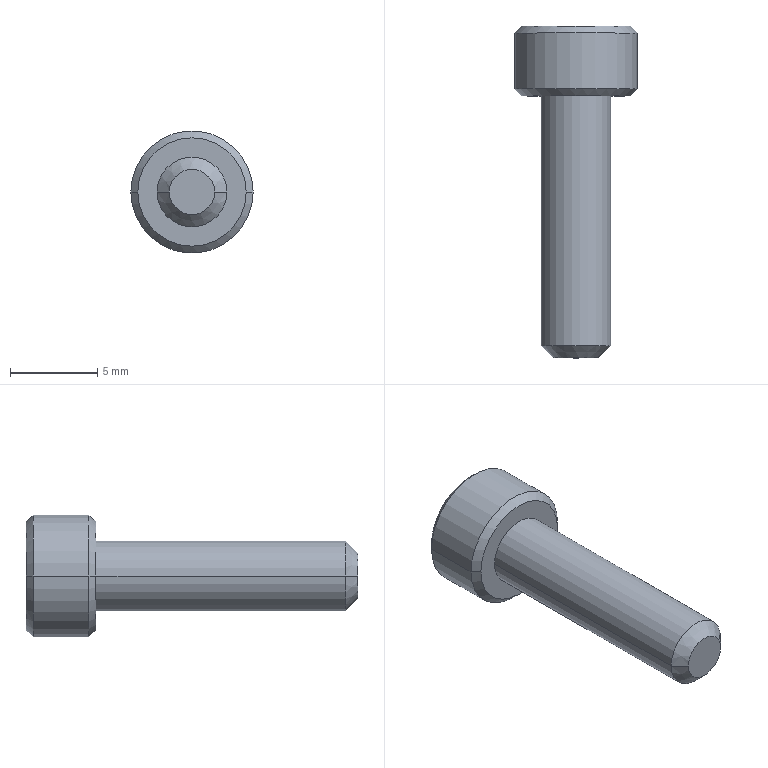Part | STEP file | BB62-M4-15L-12 | 1 solid | 27 faces | box 7 x 19 x 7 mm | volume 317.881 mm3 | plane 15 | cone 8 | cylinder 4 | commonest cylinder face diameters 4 x2 7 x2
STEP:
#1=CARTESIAN_POINT('',(0.,1.007,0.));
#2=VERTEX_POINT('',#1);
#3=CARTESIAN_POINT('',(1.72,2.,0.));
#4=VERTEX_POINT('',#3);
#5=CARTESIAN_POINT('',(0.,1.007,0.));
#6=DIRECTION('',(0.866,0.5,0.));
#7=VECTOR('',#6,1000.);
#8=LINE('',#5,#7);
#9=EDGE_CURVE('',#2,#4,#8,.T.);
#10=ORIENTED_EDGE('',*,*,#9,.F.);
#11=CARTESIAN_POINT('',(-1.72,2.,0.));
#12=VERTEX_POINT('',#11);
#13=CARTESIAN_POINT('',(0.,1.007,0.));
#14=DIRECTION('',(-0.866,0.5,0.));
#15=VECTOR('',#14,1000.);
#16=LINE('',#13,#15);
#17=EDGE_CURVE('',#2,#12,#16,.T.);
#18=ORIENTED_EDGE('',*,*,#17,.T.);
#19=CARTESIAN_POINT('',(-1.49,2.,0.86));
#20=VERTEX_POINT('',#19);
#21=CARTESIAN_POINT('',(0.,2.,0.));
#22=DIRECTION('',(0.,-1.,0.));
#23=DIRECTION('',(-1.,0.,0.));
#24=AXIS2_PLACEMENT_3D('',#21,#22,#23);
#25=CIRCLE('',#24,1.72);
#26=EDGE_CURVE('',#20,#12,#25,.T.);
#27=ORIENTED_EDGE('',*,*,#26,.F.);
#28=CARTESIAN_POINT('',(0.,2.,1.72));
#29=VERTEX_POINT('',#28);
#30=CARTESIAN_POINT('',(0.,2.,0.));
#31=DIRECTION('',(0.,-1.,0.));
#32=DIRECTION('',(-1.,0.,0.));
#33=AXIS2_PLACEMENT_3D('',#30,#31,#32);
#34=CIRCLE('',#33,1.72);
#35=EDGE_CURVE('',#29,#20,#34,.T.);
#36=ORIENTED_EDGE('',*,*,#35,.F.);
#37=CARTESIAN_POINT('',(1.49,2.,0.86));
#38=VERTEX_POINT('',#37);
#39=CARTESIAN_POINT('',(0.,2.,0.));
#40=DIRECTION('',(0.,-1.,0.));
#41=DIRECTION('',(-1.,0.,0.));
#42=AXIS2_PLACEMENT_3D('',#39,#40,#41);
#43=CIRCLE('',#42,1.72);
#44=EDGE_CURVE('',#38,#29,#43,.T.);
#45=ORIENTED_EDGE('',*,*,#44,.F.);
#46=CARTESIAN_POINT('',(0.,2.,0.));
#47=DIRECTION('',(0.,-1.,0.));
#48=DIRECTION('',(-1.,0.,0.));
#49=AXIS2_PLACEMENT_3D('',#46,#47,#48);
#50=CIRCLE('',#49,1.72);
#51=EDGE_CURVE('',#4,#38,#50,.T.);
#52=ORIENTED_EDGE('',*,*,#51,.F.);
#53=EDGE_LOOP('',(#10,#18,#27,#36,#45,#52));
#54=FACE_OUTER_BOUND('',#53,.T.);
#55=CARTESIAN_POINT('',(0.,1001.007,0.));
#56=DIRECTION('',(0.,1.,0.));
#57=DIRECTION('',(1.,0.,0.));
#58=AXIS2_PLACEMENT_3D('',#55,#56,#57);
#59=CONICAL_SURFACE('',#58,1732.051,1.047);
#60=ADVANCED_FACE('',(#54),#59,.F.);
#61=CARTESIAN_POINT('',(1.3,-15.,0.));
#62=VERTEX_POINT('',#61);
#63=CARTESIAN_POINT('',(-1.3,-15.,0.));
#64=VERTEX_POINT('',#63);
#65=CARTESIAN_POINT('',(0.,-15.,0.));
#66=DIRECTION('',(0.,1.,0.));
#67=DIRECTION('',(1.,0.,0.));
#68=AXIS2_PLACEMENT_3D('',#65,#66,#67);
#69=CIRCLE('',#68,1.3);
#70=EDGE_CURVE('',#62,#64,#69,.T.);
#71=ORIENTED_EDGE('',*,*,#70,.T.);
#72=CARTESIAN_POINT('',(-2.,-14.3,0.));
#73=VERTEX_POINT('',#72);
#74=CARTESIAN_POINT('',(-1.3,-15.,0.));
#75=DIRECTION('',(-0.7071,0.7071,0.));
#76=VECTOR('',#75,1000.);
#77=LINE('',#74,#76);
#78=EDGE_CURVE('',#64,#73,#77,.T.);
#79=ORIENTED_EDGE('',*,*,#78,.T.);
#80=CARTESIAN_POINT('',(2.,-14.3,0.));
#81=VERTEX_POINT('',#80);
#82=CARTESIAN_POINT('',(0.,-14.3,0.));
#83=DIRECTION('',(0.,-1.,0.));
#84=DIRECTION('',(-1.,0.,0.));
#85=AXIS2_PLACEMENT_3D('',#82,#83,#84);
#86=CIRCLE('',#85,2.);
#87=EDGE_CURVE('',#73,#81,#86,.T.);
#88=ORIENTED_EDGE('',*,*,#87,.T.);
#89=CARTESIAN_POINT('',(1.3,-15.,0.));
#90=DIRECTION('',(0.7071,0.7071,0.));
#91=VECTOR('',#90,1000.);
#92=LINE('',#89,#91);
#93=EDGE_CURVE('',#62,#81,#92,.T.);
#94=ORIENTED_EDGE('',*,*,#93,.F.);
#95=EDGE_LOOP('',(#71,#79,#88,#94));
#96=FACE_OUTER_BOUND('',#95,.T.);
#97=CARTESIAN_POINT('',(0.,-15.,0.));
#98=DIRECTION('',(0.,1.,0.));
#99=DIRECTION('',(1.,0.,0.));
#100=AXIS2_PLACEMENT_3D('',#97,#98,#99);
#101=CONICAL_SURFACE('',#100,1.3,0.7854);
#102=ADVANCED_FACE('',(#96),#101,.T.);
#103=ORIENTED_EDGE('',*,*,#87,.F.);
#104=CARTESIAN_POINT('',(-2.,0.,0.));
#105=VERTEX_POINT('',#104);
#106=CARTESIAN_POINT('',(-2.,-14.3,0.));
#107=DIRECTION('',(0.,1.,0.));
#108=VECTOR('',#107,1000.);
#109=LINE('',#106,#108);
#110=EDGE_CURVE('',#73,#105,#109,.T.);
#111=ORIENTED_EDGE('',*,*,#110,.T.);
#112=CARTESIAN_POINT('',(2.,0.,0.));
#113=VERTEX_POINT('',#112);
#114=CARTESIAN_POINT('',(0.,0.,0.));
#115=DIRECTION('',(0.,-1.,0.));
#116=DIRECTION('',(-1.,0.,0.));
#117=AXIS2_PLACEMENT_3D('',#114,#115,#116);
#118=CIRCLE('',#117,2.);
#119=EDGE_CURVE('',#105,#113,#118,.T.);
#120=ORIENTED_EDGE('',*,*,#119,.T.);
#121=CARTESIAN_POINT('',(2.,-14.3,0.));
#122=DIRECTION('',(0.,1.,0.));
#123=VECTOR('',#122,1000.);
#124=LINE('',#121,#123);
#125=EDGE_CURVE('',#81,#113,#124,.T.);
#126=ORIENTED_EDGE('',*,*,#125,.F.);
#127=EDGE_LOOP('',(#103,#111,#120,#126));
#128=FACE_OUTER_BOUND('',#127,.T.);
#129=CARTESIAN_POINT('',(0.,-14.3,0.));
#130=DIRECTION('',(0.,1.,0.));
#131=DIRECTION('',(1.,0.,0.));
#132=AXIS2_PLACEMENT_3D('',#129,#130,#131);
#133=CYLINDRICAL_SURFACE('',#132,2.);
#134=ADVANCED_FACE('',(#128),#133,.T.);
#135=CARTESIAN_POINT('',(-3.1,4.,0.));
#136=VERTEX_POINT('',#135);
#137=CARTESIAN_POINT('',(3.1,4.,0.));
#138=VERTEX_POINT('',#137);
#139=CARTESIAN_POINT('',(0.,4.,0.));
#140=DIRECTION('',(0.,-1.,0.));
#141=DIRECTION('',(-1.,0.,0.));
#142=AXIS2_PLACEMENT_3D('',#139,#140,#141);
#143=CIRCLE('',#142,3.1);
#144=EDGE_CURVE('',#136,#138,#143,.T.);
#145=ORIENTED_EDGE('',*,*,#144,.T.);
#146=CARTESIAN_POINT('',(3.5,3.6,0.));
#147=VERTEX_POINT('',#146);
#148=CARTESIAN_POINT('',(3.5,3.6,0.));
#149=DIRECTION('',(0.7071,-0.7071,0.));
#150=VECTOR('',#149,1000.);
#151=LINE('',#148,#150);
#152=EDGE_CURVE('',#138,#147,#151,.T.);
#153=ORIENTED_EDGE('',*,*,#152,.T.);
#154=CARTESIAN_POINT('',(-3.5,3.6,0.));
#155=VERTEX_POINT('',#154);
#156=CARTESIAN_POINT('',(0.,3.6,0.));
#157=DIRECTION('',(0.,-1.,0.));
#158=DIRECTION('',(-1.,0.,0.));
#159=AXIS2_PLACEMENT_3D('',#156,#157,#158);
#160=CIRCLE('',#159,3.5);
#161=EDGE_CURVE('',#155,#147,#160,.T.);
#162=ORIENTED_EDGE('',*,*,#161,.F.);
#163=CARTESIAN_POINT('',(-3.5,3.6,0.));
#164=DIRECTION('',(-0.7071,-0.7071,0.));
#165=VECTOR('',#164,1000.);
#166=LINE('',#163,#165);
#167=EDGE_CURVE('',#136,#155,#166,.T.);
#168=ORIENTED_EDGE('',*,*,#167,.F.);
#169=EDGE_LOOP('',(#145,#153,#162,#168));
#170=FACE_OUTER_BOUND('',#169,.T.);
#171=CARTESIAN_POINT('',(0.,3.6,0.));
#172=DIRECTION('',(0.,-1.,0.));
#173=DIRECTION('',(-1.,0.,0.));
#174=AXIS2_PLACEMENT_3D('',#171,#172,#173);
#175=CONICAL_SURFACE('',#174,3.5,0.7854);
#176=ADVANCED_FACE('',(#170),#175,.T.);
#177=ORIENTED_EDGE('',*,*,#161,.T.);
#178=CARTESIAN_POINT('',(3.5,0.4,0.));
#179=VERTEX_POINT('',#178);
#180=CARTESIAN_POINT('',(3.5,1.62,0.));
#181=DIRECTION('',(0.,-1.,0.));
#182=VECTOR('',#181,1000.);
#183=LINE('',#180,#182);
#184=EDGE_CURVE('',#147,#179,#183,.T.);
#185=ORIENTED_EDGE('',*,*,#184,.T.);
#186=CARTESIAN_POINT('',(-3.5,0.4,0.));
#187=VERTEX_POINT('',#186);
#188=CARTESIAN_POINT('',(0.,0.4,0.));
#189=DIRECTION('',(0.,-1.,0.));
#190=DIRECTION('',(-1.,0.,0.));
#191=AXIS2_PLACEMENT_3D('',#188,#189,#190);
#192=CIRCLE('',#191,3.5);
#193=EDGE_CURVE('',#187,#179,#192,.T.);
#194=ORIENTED_EDGE('',*,*,#193,.F.);
#195=CARTESIAN_POINT('',(-3.5,1.62,0.));
#196=DIRECTION('',(0.,-1.,0.));
#197=VECTOR('',#196,1000.);
#198=LINE('',#195,#197);
#199=EDGE_CURVE('',#155,#187,#198,.T.);
#200=ORIENTED_EDGE('',*,*,#199,.F.);
#201=EDGE_LOOP('',(#177,#185,#194,#200));
#202=FACE_OUTER_BOUND('',#201,.T.);
#203=CARTESIAN_POINT('',(0.,1.62,0.));
#204=DIRECTION('',(0.,-1.,0.));
#205=DIRECTION('',(-1.,0.,0.));
#206=AXIS2_PLACEMENT_3D('',#203,#204,#205);
#207=CYLINDRICAL_SURFACE('',#206,3.5);
#208=ADVANCED_FACE('',(#202),#207,.T.);
#209=CARTESIAN_POINT('',(-3.1,0.,0.));
#210=VERTEX_POINT('',#209);
#211=CARTESIAN_POINT('',(3.1,0.,0.));
#212=VERTEX_POINT('',#211);
#213=CARTESIAN_POINT('',(0.,0.,0.));
#214=DIRECTION('',(0.,-1.,0.));
#215=DIRECTION('',(-1.,0.,0.));
#216=AXIS2_PLACEMENT_3D('',#213,#214,#215);
#217=CIRCLE('',#216,3.1);
#218=EDGE_CURVE('',#210,#212,#217,.T.);
#219=ORIENTED_EDGE('',*,*,#218,.F.);
#220=CARTESIAN_POINT('',(-3.1,0.,0.));
#221=DIRECTION('',(-0.7071,0.7071,0.));
#222=VECTOR('',#221,1000.);
#223=LINE('',#220,#222);
#224=EDGE_CURVE('',#210,#187,#223,.T.);
#225=ORIENTED_EDGE('',*,*,#224,.T.);
#226=ORIENTED_EDGE('',*,*,#193,.T.);
#227=CARTESIAN_POINT('',(3.1,0.,0.));
#228=DIRECTION('',(0.7071,0.7071,0.));
#229=VECTOR('',#228,1000.);
#230=LINE('',#227,#229);
#231=EDGE_CURVE('',#212,#179,#230,.T.);
#232=ORIENTED_EDGE('',*,*,#231,.F.);
#233=EDGE_LOOP('',(#219,#225,#226,#232));
#234=FACE_OUTER_BOUND('',#233,.T.);
#235=CARTESIAN_POINT('',(0.,0.,0.));
#236=DIRECTION('',(0.,1.,0.));
#237=DIRECTION('',(1.,0.,0.));
#238=AXIS2_PLACEMENT_3D('',#235,#236,#237);
#239=CONICAL_SURFACE('',#238,3.1,0.7854);
#240=ADVANCED_FACE('',(#234),#239,.T.);
#241=ORIENTED_EDGE('',*,*,#144,.F.);
#242=CARTESIAN_POINT('',(0.,4.,0.));
#243=DIRECTION('',(0.,-1.,0.));
#244=DIRECTION('',(-1.,0.,0.));
#245=AXIS2_PLACEMENT_3D('',#242,#243,#244);
#246=CIRCLE('',#245,3.1);
#247=EDGE_CURVE('',#138,#136,#246,.T.);
#248=ORIENTED_EDGE('',*,*,#247,.F.);
#249=EDGE_LOOP('',(#241,#248));
#250=FACE_OUTER_BOUND('',#249,.T.);
#251=CARTESIAN_POINT('',(0.,4.,-1.72));
#252=VERTEX_POINT('',#251);
#253=CARTESIAN_POINT('',(-1.49,4.,-0.86));
#254=VERTEX_POINT('',#253);
#255=CARTESIAN_POINT('',(0.,4.,-1.72));
#256=DIRECTION('',(-0.866,0.,0.5));
#257=VECTOR('',#256,1000.);
#258=LINE('',#255,#257);
#259=EDGE_CURVE('',#252,#254,#258,.T.);
#260=ORIENTED_EDGE('',*,*,#259,.F.);
#261=CARTESIAN_POINT('',(1.49,4.,-0.86));
#262=VERTEX_POINT('',#261);
#263=CARTESIAN_POINT('',(1.49,4.,-0.86));
#264=DIRECTION('',(-0.866,0.,-0.5));
#265=VECTOR('',#264,1000.);
#266=LINE('',#263,#265);
#267=EDGE_CURVE('',#262,#252,#266,.T.);
#268=ORIENTED_EDGE('',*,*,#267,.F.);
#269=CARTESIAN_POINT('',(1.49,4.,0.86));
#270=VERTEX_POINT('',#269);
#271=CARTESIAN_POINT('',(1.49,4.,0.86));
#272=DIRECTION('',(0.,0.,-1.));
#273=VECTOR('',#272,1000.);
#274=LINE('',#271,#273);
#275=EDGE_CURVE('',#270,#262,#274,.T.);
#276=ORIENTED_EDGE('',*,*,#275,.F.);
#277=CARTESIAN_POINT('',(0.,4.,1.72));
#278=VERTEX_POINT('',#277);
#279=CARTESIAN_POINT('',(0.,4.,1.72));
#280=DIRECTION('',(0.866,0.,-0.5));
#281=VECTOR('',#280,1000.);
#282=LINE('',#279,#281);
#283=EDGE_CURVE('',#278,#270,#282,.T.);
#284=ORIENTED_EDGE('',*,*,#283,.F.);
#285=CARTESIAN_POINT('',(-1.49,4.,0.86));
#286=VERTEX_POINT('',#285);
#287=CARTESIAN_POINT('',(-1.49,4.,0.86));
#288=DIRECTION('',(0.866,0.,0.5));
#289=VECTOR('',#288,1000.);
#290=LINE('',#287,#289);
#291=EDGE_CURVE('',#286,#278,#290,.T.);
#292=ORIENTED_EDGE('',*,*,#291,.F.);
#293=CARTESIAN_POINT('',(-1.49,4.,-0.86));
#294=DIRECTION('',(0.,0.,1.));
#295=VECTOR('',#294,1000.);
#296=LINE('',#293,#295);
#297=EDGE_CURVE('',#254,#286,#296,.T.);
#298=ORIENTED_EDGE('',*,*,#297,.F.);
#299=EDGE_LOOP('',(#260,#268,#276,#284,#292,#298));
#300=FACE_BOUND('',#299,.T.);
#301=CARTESIAN_POINT('',(3.1,4.,0.));
#302=DIRECTION('',(0.,1.,0.));
#303=DIRECTION('',(1.,0.,0.));
#304=AXIS2_PLACEMENT_3D('',#301,#302,#303);
#305=PLANE('',#304);
#306=ADVANCED_FACE('',(#250,#300),#305,.T.);
#307=CARTESIAN_POINT('',(0.,0.,0.));
#308=DIRECTION('',(0.,-1.,0.));
#309=DIRECTION('',(-1.,0.,0.));
#310=AXIS2_PLACEMENT_3D('',#307,#308,#309);
#311=CIRCLE('',#310,2.);
#312=EDGE_CURVE('',#113,#105,#311,.T.);
#313=ORIENTED_EDGE('',*,*,#312,.F.);
#314=ORIENTED_EDGE('',*,*,#119,.F.);
#315=EDGE_LOOP('',(#313,#314));
#316=FACE_BOUND('',#315,.T.);
#317=CARTESIAN_POINT('',(0.,0.,0.));
#318=DIRECTION('',(0.,-1.,0.));
#319=DIRECTION('',(-1.,0.,0.));
#320=AXIS2_PLACEMENT_3D('',#317,#318,#319);
#321=CIRCLE('',#320,3.1);
#322=EDGE_CURVE('',#212,#210,#321,.T.);
#323=ORIENTED_EDGE('',*,*,#322,.T.);
#324=ORIENTED_EDGE('',*,*,#218,.T.);
#325=EDGE_LOOP('',(#323,#324));
#326=FACE_OUTER_BOUND('',#325,.T.);
#327=CARTESIAN_POINT('',(0.,0.,0.));
#328=DIRECTION('',(0.,-1.,0.));
#329=DIRECTION('',(-1.,0.,0.));
#330=AXIS2_PLACEMENT_3D('',#327,#328,#329);
#331=PLANE('',#330);
#332=ADVANCED_FACE('',(#316,#326),#331,.T.);
#333=ORIENTED_EDGE('',*,*,#224,.F.);
#334=ORIENTED_EDGE('',*,*,#322,.F.);
#335=ORIENTED_EDGE('',*,*,#231,.T.);
#336=CARTESIAN_POINT('',(0.,0.4,0.));
#337=DIRECTION('',(0.,-1.,0.));
#338=DIRECTION('',(-1.,0.,0.));
#339=AXIS2_PLACEMENT_3D('',#336,#337,#338);
#340=CIRCLE('',#339,3.5);
#341=EDGE_CURVE('',#179,#187,#340,.T.);
#342=ORIENTED_EDGE('',*,*,#341,.T.);
#343=EDGE_LOOP('',(#333,#334,#335,#342));
#344=FACE_OUTER_BOUND('',#343,.T.);
#345=CARTESIAN_POINT('',(0.,0.,0.));
#346=DIRECTION('',(0.,1.,0.));
#347=DIRECTION('',(1.,0.,0.));
#348=AXIS2_PLACEMENT_3D('',#345,#346,#347);
#349=CONICAL_SURFACE('',#348,3.1,0.7854);
#350=ADVANCED_FACE('',(#344),#349,.T.);
#351=ORIENTED_EDGE('',*,*,#184,.F.);
#352=CARTESIAN_POINT('',(0.,3.6,0.));
#353=DIRECTION('',(0.,-1.,0.));
#354=DIRECTION('',(-1.,0.,0.));
#355=AXIS2_PLACEMENT_3D('',#352,#353,#354);
#356=CIRCLE('',#355,3.5);
#357=EDGE_CURVE('',#147,#155,#356,.T.);
#358=ORIENTED_EDGE('',*,*,#357,.T.);
#359=ORIENTED_EDGE('',*,*,#199,.T.);
#360=ORIENTED_EDGE('',*,*,#341,.F.);
#361=EDGE_LOOP('',(#351,#358,#359,#360));
#362=FACE_OUTER_BOUND('',#361,.T.);
#363=CARTESIAN_POINT('',(0.,1.62,0.));
#364=DIRECTION('',(0.,-1.,0.));
#365=DIRECTION('',(-1.,0.,0.));
#366=AXIS2_PLACEMENT_3D('',#363,#364,#365);
#367=CYLINDRICAL_SURFACE('',#366,3.5);
#368=ADVANCED_FACE('',(#362),#367,.T.);
#369=ORIENTED_EDGE('',*,*,#152,.F.);
#370=ORIENTED_EDGE('',*,*,#247,.T.);
#371=ORIENTED_EDGE('',*,*,#167,.T.);
#372=ORIENTED_EDGE('',*,*,#357,.F.);
#373=EDGE_LOOP('',(#369,#370,#371,#372));
#374=FACE_OUTER_BOUND('',#373,.T.);
#375=CARTESIAN_POINT('',(0.,3.6,0.));
#376=DIRECTION('',(0.,-1.,0.));
#377=DIRECTION('',(-1.,0.,0.));
#378=AXIS2_PLACEMENT_3D('',#375,#376,#377);
#379=CONICAL_SURFACE('',#378,3.5,0.7854);
#380=ADVANCED_FACE('',(#374),#379,.T.);
#381=ORIENTED_EDGE('',*,*,#110,.F.);
#382=CARTESIAN_POINT('',(0.,-14.3,0.));
#383=DIRECTION('',(0.,-1.,0.));
#384=DIRECTION('',(-1.,0.,0.));
#385=AXIS2_PLACEMENT_3D('',#382,#383,#384);
#386=CIRCLE('',#385,2.);
#387=EDGE_CURVE('',#81,#73,#386,.T.);
#388=ORIENTED_EDGE('',*,*,#387,.F.);
#389=ORIENTED_EDGE('',*,*,#125,.T.);
#390=ORIENTED_EDGE('',*,*,#312,.T.);
#391=EDGE_LOOP('',(#381,#388,#389,#390));
#392=FACE_OUTER_BOUND('',#391,.T.);
#393=CARTESIAN_POINT('',(0.,-14.3,0.));
#394=DIRECTION('',(0.,1.,0.));
#395=DIRECTION('',(1.,0.,0.));
#396=AXIS2_PLACEMENT_3D('',#393,#394,#395);
#397=CYLINDRICAL_SURFACE('',#396,2.);
#398=ADVANCED_FACE('',(#392),#397,.T.);
#399=ORIENTED_EDGE('',*,*,#70,.F.);
#400=CARTESIAN_POINT('',(0.,-15.,0.));
#401=DIRECTION('',(0.,1.,0.));
#402=DIRECTION('',(1.,0.,0.));
#403=AXIS2_PLACEMENT_3D('',#400,#401,#402);
#404=CIRCLE('',#403,1.3);
#405=EDGE_CURVE('',#64,#62,#404,.T.);
#406=ORIENTED_EDGE('',*,*,#405,.F.);
#407=EDGE_LOOP('',(#399,#406));
#408=FACE_OUTER_BOUND('',#407,.T.);
#409=CARTESIAN_POINT('',(0.,-15.,0.));
#410=DIRECTION('',(0.,-1.,0.));
#411=DIRECTION('',(-1.,0.,0.));
#412=AXIS2_PLACEMENT_3D('',#409,#410,#411);
#413=PLANE('',#412);
#414=ADVANCED_FACE('',(#408),#413,.T.);
#415=ORIENTED_EDGE('',*,*,#78,.F.);
#416=ORIENTED_EDGE('',*,*,#405,.T.);
#417=ORIENTED_EDGE('',*,*,#93,.T.);
#418=ORIENTED_EDGE('',*,*,#387,.T.);
#419=EDGE_LOOP('',(#415,#416,#417,#418));
#420=FACE_OUTER_BOUND('',#419,.T.);
#421=CARTESIAN_POINT('',(0.,-15.,0.));
#422=DIRECTION('',(0.,1.,0.));
#423=DIRECTION('',(1.,0.,0.));
#424=AXIS2_PLACEMENT_3D('',#421,#422,#423);
#425=CONICAL_SURFACE('',#424,1.3,0.7854);
#426=ADVANCED_FACE('',(#420),#425,.T.);
#427=CARTESIAN_POINT('',(1.49,2.,-0.86));
#428=VERTEX_POINT('',#427);
#429=CARTESIAN_POINT('',(0.,2.,-1.72));
#430=VERTEX_POINT('',#429);
#431=CARTESIAN_POINT('',(1.49,2.,-0.86));
#432=DIRECTION('',(-0.866,0.,-0.5));
#433=VECTOR('',#432,1000.);
#434=LINE('',#431,#433);
#435=EDGE_CURVE('',#428,#430,#434,.T.);
#436=ORIENTED_EDGE('',*,*,#435,.F.);
#437=CARTESIAN_POINT('',(1.49,4.,-0.86));
#438=DIRECTION('',(0.,-1.,0.));
#439=VECTOR('',#438,1000.);
#440=LINE('',#437,#439);
#441=EDGE_CURVE('',#262,#428,#440,.T.);
#442=ORIENTED_EDGE('',*,*,#441,.F.);
#443=ORIENTED_EDGE('',*,*,#267,.T.);
#444=CARTESIAN_POINT('',(0.,4.,-1.72));
#445=DIRECTION('',(0.,-1.,0.));
#446=VECTOR('',#445,1000.);
#447=LINE('',#444,#446);
#448=EDGE_CURVE('',#252,#430,#447,.T.);
#449=ORIENTED_EDGE('',*,*,#448,.T.);
#450=EDGE_LOOP('',(#436,#442,#443,#449));
#451=FACE_OUTER_BOUND('',#450,.T.);
#452=CARTESIAN_POINT('',(1.49,4.,-0.86));
#453=DIRECTION('',(-0.5,0.,0.866));
#454=DIRECTION('',(0.866,0.,0.5));
#455=AXIS2_PLACEMENT_3D('',#452,#453,#454);
#456=PLANE('',#455);
#457=ADVANCED_FACE('',(#451),#456,.T.);
#458=CARTESIAN_POINT('',(-1.49,2.,-0.86));
#459=VERTEX_POINT('',#458);
#460=CARTESIAN_POINT('',(0.,2.,-1.72));
#461=DIRECTION('',(-0.866,0.,0.5));
#462=VECTOR('',#461,1000.);
#463=LINE('',#460,#462);
#464=EDGE_CURVE('',#430,#459,#463,.T.);
#465=ORIENTED_EDGE('',*,*,#464,.F.);
#466=ORIENTED_EDGE('',*,*,#448,.F.);
#467=ORIENTED_EDGE('',*,*,#259,.T.);
#468=CARTESIAN_POINT('',(-1.49,4.,-0.86));
#469=DIRECTION('',(0.,-1.,0.));
#470=VECTOR('',#469,1000.);
#471=LINE('',#468,#470);
#472=EDGE_CURVE('',#254,#459,#471,.T.);
#473=ORIENTED_EDGE('',*,*,#472,.T.);
#474=EDGE_LOOP('',(#465,#466,#467,#473));
#475=FACE_OUTER_BOUND('',#474,.T.);
#476=CARTESIAN_POINT('',(0.,4.,-1.72));
#477=DIRECTION('',(0.5,0.,0.866));
#478=DIRECTION('',(0.866,0.,-0.5));
#479=AXIS2_PLACEMENT_3D('',#476,#477,#478);
#480=PLANE('',#479);
#481=ADVANCED_FACE('',(#475),#480,.T.);
#482=CARTESIAN_POINT('',(-1.49,2.,-0.86));
#483=DIRECTION('',(0.,0.,1.));
#484=VECTOR('',#483,1000.);
#485=LINE('',#482,#484);
#486=EDGE_CURVE('',#459,#20,#485,.T.);
#487=ORIENTED_EDGE('',*,*,#486,.F.);
#488=ORIENTED_EDGE('',*,*,#472,.F.);
#489=ORIENTED_EDGE('',*,*,#297,.T.);
#490=CARTESIAN_POINT('',(-1.49,4.,0.86));
#491=DIRECTION('',(0.,-1.,0.));
#492=VECTOR('',#491,1000.);
#493=LINE('',#490,#492);
#494=EDGE_CURVE('',#286,#20,#493,.T.);
#495=ORIENTED_EDGE('',*,*,#494,.T.);
#496=EDGE_LOOP('',(#487,#488,#489,#495));
#497=FACE_OUTER_BOUND('',#496,.T.);
#498=CARTESIAN_POINT('',(-1.49,4.,-0.86));
#499=DIRECTION('',(1.,0.,0.));
#500=DIRECTION('',(0.,0.,-1.));
#501=AXIS2_PLACEMENT_3D('',#498,#499,#500);
#502=PLANE('',#501);
#503=ADVANCED_FACE('',(#497),#502,.T.);
#504=CARTESIAN_POINT('',(-1.49,2.,0.86));
#505=DIRECTION('',(0.866,0.,0.5));
#506=VECTOR('',#505,1000.);
#507=LINE('',#504,#506);
#508=EDGE_CURVE('',#20,#29,#507,.T.);
#509=ORIENTED_EDGE('',*,*,#508,.F.);
#510=ORIENTED_EDGE('',*,*,#494,.F.);
#511=ORIENTED_EDGE('',*,*,#291,.T.);
#512=CARTESIAN_POINT('',(0.,4.,1.72));
#513=DIRECTION('',(0.,-1.,0.));
#514=VECTOR('',#513,1000.);
#515=LINE('',#512,#514);
#516=EDGE_CURVE('',#278,#29,#515,.T.);
#517=ORIENTED_EDGE('',*,*,#516,.T.);
#518=EDGE_LOOP('',(#509,#510,#511,#517));
#519=FACE_OUTER_BOUND('',#518,.T.);
#520=CARTESIAN_POINT('',(-1.49,4.,0.86));
#521=DIRECTION('',(0.5,0.,-0.866));
#522=DIRECTION('',(-0.866,0.,-0.5));
#523=AXIS2_PLACEMENT_3D('',#520,#521,#522);
#524=PLANE('',#523);
#525=ADVANCED_FACE('',(#519),#524,.T.);
#526=CARTESIAN_POINT('',(0.,2.,1.72));
#527=DIRECTION('',(0.866,0.,-0.5));
#528=VECTOR('',#527,1000.);
#529=LINE('',#526,#528);
#530=EDGE_CURVE('',#29,#38,#529,.T.);
#531=ORIENTED_EDGE('',*,*,#530,.F.);
#532=ORIENTED_EDGE('',*,*,#516,.F.);
#533=ORIENTED_EDGE('',*,*,#283,.T.);
#534=CARTESIAN_POINT('',(1.49,4.,0.86));
#535=DIRECTION('',(0.,-1.,0.));
#536=VECTOR('',#535,1000.);
#537=LINE('',#534,#536);
#538=EDGE_CURVE('',#270,#38,#537,.T.);
#539=ORIENTED_EDGE('',*,*,#538,.T.);
#540=EDGE_LOOP('',(#531,#532,#533,#539));
#541=FACE_OUTER_BOUND('',#540,.T.);
#542=CARTESIAN_POINT('',(0.,4.,1.72));
#543=DIRECTION('',(-0.5,0.,-0.866));
#544=DIRECTION('',(-0.866,0.,0.5));
#545=AXIS2_PLACEMENT_3D('',#542,#543,#544);
#546=PLANE('',#545);
#547=ADVANCED_FACE('',(#541),#546,.T.);
#548=CARTESIAN_POINT('',(1.49,2.,0.86));
#549=DIRECTION('',(0.,0.,-1.));
#550=VECTOR('',#549,1000.);
#551=LINE('',#548,#550);
#552=EDGE_CURVE('',#38,#428,#551,.T.);
#553=ORIENTED_EDGE('',*,*,#552,.F.);
#554=ORIENTED_EDGE('',*,*,#538,.F.);
#555=ORIENTED_EDGE('',*,*,#275,.T.);
#556=ORIENTED_EDGE('',*,*,#441,.T.);
#557=EDGE_LOOP('',(#553,#554,#555,#556));
#558=FACE_OUTER_BOUND('',#557,.T.);
#559=CARTESIAN_POINT('',(1.49,4.,0.86));
#560=DIRECTION('',(-1.,0.,0.));
#561=DIRECTION('',(0.,0.,1.));
#562=AXIS2_PLACEMENT_3D('',#559,#560,#561);
#563=PLANE('',#562);
#564=ADVANCED_FACE('',(#558),#563,.T.);
#565=ORIENTED_EDGE('',*,*,#435,.T.);
#566=CARTESIAN_POINT('',(0.,2.,0.));
#567=DIRECTION('',(0.,-1.,0.));
#568=DIRECTION('',(-1.,0.,0.));
#569=AXIS2_PLACEMENT_3D('',#566,#567,#568);
#570=CIRCLE('',#569,1.72);
#571=EDGE_CURVE('',#430,#428,#570,.T.);
#572=ORIENTED_EDGE('',*,*,#571,.T.);
#573=EDGE_LOOP('',(#565,#572));
#574=FACE_OUTER_BOUND('',#573,.T.);
#575=CARTESIAN_POINT('',(0.,2.,0.));
#576=DIRECTION('',(0.,1.,0.));
#577=DIRECTION('',(1.,0.,0.));
#578=AXIS2_PLACEMENT_3D('',#575,#576,#577);
#579=PLANE('',#578);
#580=ADVANCED_FACE('',(#574),#579,.F.);
#581=ORIENTED_EDGE('',*,*,#552,.T.);
#582=CARTESIAN_POINT('',(0.,2.,0.));
#583=DIRECTION('',(0.,-1.,0.));
#584=DIRECTION('',(-1.,0.,0.));
#585=AXIS2_PLACEMENT_3D('',#582,#583,#584);
#586=CIRCLE('',#585,1.72);
#587=EDGE_CURVE('',#428,#4,#586,.T.);
#588=ORIENTED_EDGE('',*,*,#587,.T.);
#589=ORIENTED_EDGE('',*,*,#51,.T.);
#590=EDGE_LOOP('',(#581,#588,#589));
#591=FACE_OUTER_BOUND('',#590,.T.);
#592=CARTESIAN_POINT('',(0.,2.,0.));
#593=DIRECTION('',(0.,1.,0.));
#594=DIRECTION('',(1.,0.,0.));
#595=AXIS2_PLACEMENT_3D('',#592,#593,#594);
#596=PLANE('',#595);
#597=ADVANCED_FACE('',(#591),#596,.F.);
#598=ORIENTED_EDGE('',*,*,#530,.T.);
#599=ORIENTED_EDGE('',*,*,#44,.T.);
#600=EDGE_LOOP('',(#598,#599));
#601=FACE_OUTER_BOUND('',#600,.T.);
#602=CARTESIAN_POINT('',(0.,2.,0.));
#603=DIRECTION('',(0.,1.,0.));
#604=DIRECTION('',(1.,0.,0.));
#605=AXIS2_PLACEMENT_3D('',#602,#603,#604);
#606=PLANE('',#605);
#607=ADVANCED_FACE('',(#601),#606,.F.);
#608=ORIENTED_EDGE('',*,*,#508,.T.);
#609=ORIENTED_EDGE('',*,*,#35,.T.);
#610=EDGE_LOOP('',(#608,#609));
#611=FACE_OUTER_BOUND('',#610,.T.);
#612=CARTESIAN_POINT('',(0.,2.,0.));
#613=DIRECTION('',(0.,1.,0.));
#614=DIRECTION('',(1.,0.,0.));
#615=AXIS2_PLACEMENT_3D('',#612,#613,#614);
#616=PLANE('',#615);
#617=ADVANCED_FACE('',(#611),#616,.F.);
#618=ORIENTED_EDGE('',*,*,#486,.T.);
#619=ORIENTED_EDGE('',*,*,#26,.T.);
#620=CARTESIAN_POINT('',(0.,2.,0.));
#621=DIRECTION('',(0.,-1.,0.));
#622=DIRECTION('',(-1.,0.,0.));
#623=AXIS2_PLACEMENT_3D('',#620,#621,#622);
#624=CIRCLE('',#623,1.72);
#625=EDGE_CURVE('',#12,#459,#624,.T.);
#626=ORIENTED_EDGE('',*,*,#625,.T.);
#627=EDGE_LOOP('',(#618,#619,#626));
#628=FACE_OUTER_BOUND('',#627,.T.);
#629=CARTESIAN_POINT('',(0.,2.,0.));
#630=DIRECTION('',(0.,1.,0.));
#631=DIRECTION('',(1.,0.,0.));
#632=AXIS2_PLACEMENT_3D('',#629,#630,#631);
#633=PLANE('',#632);
#634=ADVANCED_FACE('',(#628),#633,.F.);
#635=ORIENTED_EDGE('',*,*,#464,.T.);
#636=CARTESIAN_POINT('',(0.,2.,0.));
#637=DIRECTION('',(0.,-1.,0.));
#638=DIRECTION('',(-1.,0.,0.));
#639=AXIS2_PLACEMENT_3D('',#636,#637,#638);
#640=CIRCLE('',#639,1.72);
#641=EDGE_CURVE('',#459,#430,#640,.T.);
#642=ORIENTED_EDGE('',*,*,#641,.T.);
#643=EDGE_LOOP('',(#635,#642));
#644=FACE_OUTER_BOUND('',#643,.T.);
#645=CARTESIAN_POINT('',(0.,2.,0.));
#646=DIRECTION('',(0.,1.,0.));
#647=DIRECTION('',(1.,0.,0.));
#648=AXIS2_PLACEMENT_3D('',#645,#646,#647);
#649=PLANE('',#648);
#650=ADVANCED_FACE('',(#644),#649,.F.);
#651=ORIENTED_EDGE('',*,*,#17,.F.);
#652=ORIENTED_EDGE('',*,*,#9,.T.);
#653=ORIENTED_EDGE('',*,*,#587,.F.);
#654=ORIENTED_EDGE('',*,*,#571,.F.);
#655=ORIENTED_EDGE('',*,*,#641,.F.);
#656=ORIENTED_EDGE('',*,*,#625,.F.);
#657=EDGE_LOOP('',(#651,#652,#653,#654,#655,#656));
#658=FACE_OUTER_BOUND('',#657,.T.);
#659=CARTESIAN_POINT('',(0.,1001.007,0.));
#660=DIRECTION('',(0.,1.,0.));
#661=DIRECTION('',(1.,0.,0.));
#662=AXIS2_PLACEMENT_3D('',#659,#660,#661);
#663=CONICAL_SURFACE('',#662,1732.051,1.047);
#664=ADVANCED_FACE('',(#658),#663,.F.);
#665=CLOSED_SHELL('',(#60,#102,#134,#176,#208,#240,#306,#332,#350,#368,#380,#398,#414,#426,#457,#481,#503,#525,#547,#564,#580,#597,#607,#617,#634,#650,#664));
#666=MANIFOLD_SOLID_BREP('',#665);
#667=CARTESIAN_POINT('',(0.,0.,0.));
#668=DIRECTION('',(0.,0.,1.));
#669=DIRECTION('',(1.,0.,0.));
#670=AXIS2_PLACEMENT_3D('',#667,#668,#669);
#671=(LENGTH_UNIT()NAMED_UNIT(*)SI_UNIT(.MILLI.,.METRE.));
#672=UNCERTAINTY_MEASURE_WITH_UNIT(LENGTH_MEASURE(0.00001),#671,'','');
#673=(NAMED_UNIT(*)PLANE_ANGLE_UNIT()SI_UNIT($,.RADIAN.));
#674=(NAMED_UNIT(*)SI_UNIT($,.STERADIAN.)SOLID_ANGLE_UNIT());
#675=(GEOMETRIC_REPRESENTATION_CONTEXT(3)GLOBAL_UNCERTAINTY_ASSIGNED_CONTEXT((#672))GLOBAL_UNIT_ASSIGNED_CONTEXT((#671,#673,#674))REPRESENTATION_CONTEXT('',''));
#676=ADVANCED_BREP_SHAPE_REPRESENTATION('',(#666,#670),#675);